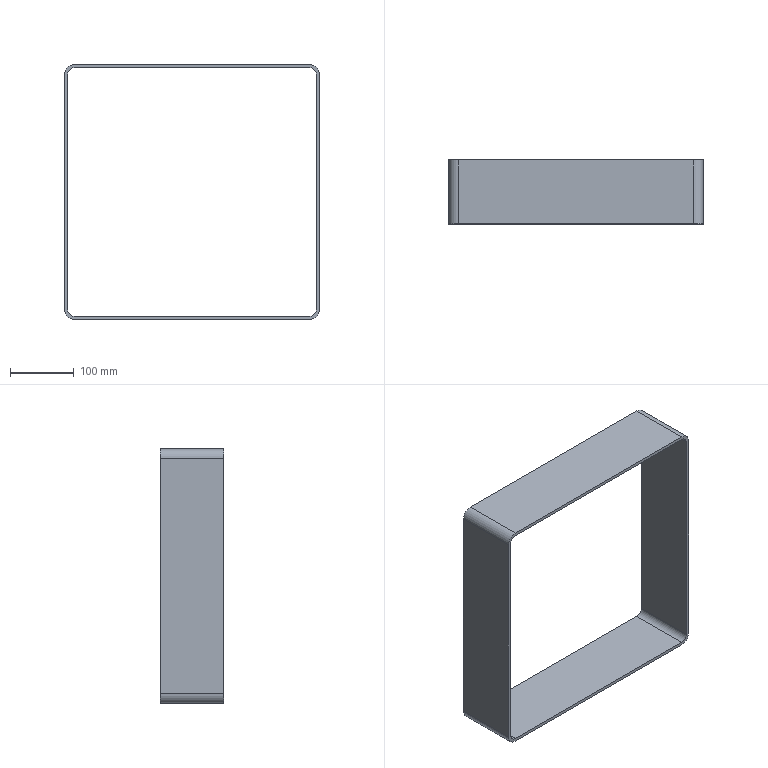Part | STEP file | Input 36 | 1 solid | 18 faces | box 400 x 100 x 400 mm | volume 779270 mm3 | plane 10 | cylinder 8 | commonest cylinder face diameters 20 x4 30 x4
STEP:
#1=CARTESIAN_POINT('',(0.,0.,0.));
#2=DIRECTION('',(0.,0.,1.));
#3=DIRECTION('',(1.,0.,0.));
#4=AXIS2_PLACEMENT_3D('',#1,#2,#3);
#5=CARTESIAN_POINT('',(-3055.,374.5,200.));
#6=VERTEX_POINT('',#5);
#7=CARTESIAN_POINT('',(-3040.,374.5,185.));
#8=VERTEX_POINT('',#7);
#9=CARTESIAN_POINT('',(-3055.,374.5,185.));
#10=DIRECTION('',(0.,1.,0.));
#11=DIRECTION('',(0.,0.,1.));
#12=AXIS2_PLACEMENT_3D('',#9,#10,#11);
#13=CIRCLE('',#12,15.);
#14=CARTESIAN_POINT('',(-3055.,374.5,185.));
#15=DIRECTION('',(0.,1.,0.));
#16=DIRECTION('',(0.,0.,1.));
#17=AXIS2_PLACEMENT_3D('',#14,#15,#16);
#18=PLANE('',#17);
#19=CARTESIAN_POINT('',(0.,0.));
#20=DIRECTION('',(1.,0.));
#21=AXIS2_PLACEMENT_2D('',#19,#20);
#22=CIRCLE('',#21,15.);
#23=(GEOMETRIC_REPRESENTATION_CONTEXT(2)PARAMETRIC_REPRESENTATION_CONTEXT()REPRESENTATION_CONTEXT('',''));
#24=DEFINITIONAL_REPRESENTATION('',(#22),#23);
#25=PCURVE('',#18,#24);
#26=CARTESIAN_POINT('',(-3055.,374.5,185.));
#27=DIRECTION('',(0.,-1.,0.));
#28=DIRECTION('',(0.,0.,-1.));
#29=AXIS2_PLACEMENT_3D('',#26,#27,#28);
#30=CYLINDRICAL_SURFACE('',#29,15.);
#31=CARTESIAN_POINT('',(3.142,0.));
#32=DIRECTION('',(-1.,0.));
#33=VECTOR('',#32,1.);
#34=LINE('',#31,#33);
#35=(GEOMETRIC_REPRESENTATION_CONTEXT(2)PARAMETRIC_REPRESENTATION_CONTEXT()REPRESENTATION_CONTEXT('',''));
#36=DEFINITIONAL_REPRESENTATION('',(#34),#35);
#37=PCURVE('',#30,#36);
#38=SURFACE_CURVE('',#13,(#25,#37),.PCURVE_S1.);
#39=EDGE_CURVE('',#6,#8,#38,.T.);
#40=ORIENTED_EDGE('',*,*,#39,.T.);
#41=CARTESIAN_POINT('',(-3040.,374.5,-185.));
#42=VERTEX_POINT('',#41);
#43=CARTESIAN_POINT('',(-3040.,374.5,185.));
#44=DIRECTION('',(0.,0.,-1.));
#45=VECTOR('',#44,1.);
#46=LINE('',#43,#45);
#47=CARTESIAN_POINT('',(0.,15.));
#48=DIRECTION('',(-1.,0.));
#49=VECTOR('',#48,1.);
#50=LINE('',#47,#49);
#51=(GEOMETRIC_REPRESENTATION_CONTEXT(2)PARAMETRIC_REPRESENTATION_CONTEXT()REPRESENTATION_CONTEXT('',''));
#52=DEFINITIONAL_REPRESENTATION('',(#50),#51);
#53=PCURVE('',#18,#52);
#54=CARTESIAN_POINT('',(-3040.,374.5,185.));
#55=DIRECTION('',(-1.,0.,0.));
#56=DIRECTION('',(0.,0.,1.));
#57=AXIS2_PLACEMENT_3D('',#54,#55,#56);
#58=PLANE('',#57);
#59=CARTESIAN_POINT('',(0.,0.));
#60=DIRECTION('',(-1.,0.));
#61=VECTOR('',#60,1.);
#62=LINE('',#59,#61);
#63=(GEOMETRIC_REPRESENTATION_CONTEXT(2)PARAMETRIC_REPRESENTATION_CONTEXT()REPRESENTATION_CONTEXT('',''));
#64=DEFINITIONAL_REPRESENTATION('',(#62),#63);
#65=PCURVE('',#58,#64);
#66=SURFACE_CURVE('',#46,(#53,#65),.PCURVE_S1.);
#67=EDGE_CURVE('',#8,#42,#66,.T.);
#68=ORIENTED_EDGE('',*,*,#67,.T.);
#69=CARTESIAN_POINT('',(-3055.,374.5,-200.));
#70=VERTEX_POINT('',#69);
#71=CARTESIAN_POINT('',(-3055.,374.5,-185.));
#72=DIRECTION('',(0.,1.,0.));
#73=DIRECTION('',(0.,0.,-1.));
#74=AXIS2_PLACEMENT_3D('',#71,#72,#73);
#75=CIRCLE('',#74,15.);
#76=CARTESIAN_POINT('',(-370.,0.));
#77=DIRECTION('',(-1.,0.));
#78=AXIS2_PLACEMENT_2D('',#76,#77);
#79=CIRCLE('',#78,15.);
#80=(GEOMETRIC_REPRESENTATION_CONTEXT(2)PARAMETRIC_REPRESENTATION_CONTEXT()REPRESENTATION_CONTEXT('',''));
#81=DEFINITIONAL_REPRESENTATION('',(#79),#80);
#82=PCURVE('',#18,#81);
#83=CARTESIAN_POINT('',(-3055.,374.5,-185.));
#84=DIRECTION('',(0.,-1.,0.));
#85=DIRECTION('',(0.,0.,-1.));
#86=AXIS2_PLACEMENT_3D('',#83,#84,#85);
#87=CYLINDRICAL_SURFACE('',#86,15.);
#88=CARTESIAN_POINT('',(6.283,0.));
#89=DIRECTION('',(-1.,0.));
#90=VECTOR('',#89,1.);
#91=LINE('',#88,#90);
#92=(GEOMETRIC_REPRESENTATION_CONTEXT(2)PARAMETRIC_REPRESENTATION_CONTEXT()REPRESENTATION_CONTEXT('',''));
#93=DEFINITIONAL_REPRESENTATION('',(#91),#92);
#94=PCURVE('',#87,#93);
#95=SURFACE_CURVE('',#75,(#82,#94),.PCURVE_S1.);
#96=EDGE_CURVE('',#42,#70,#95,.T.);
#97=ORIENTED_EDGE('',*,*,#96,.T.);
#98=CARTESIAN_POINT('',(-3425.,374.5,-200.));
#99=VERTEX_POINT('',#98);
#100=CARTESIAN_POINT('',(-3425.,374.5,-200.));
#101=DIRECTION('',(-1.,0.,0.));
#102=VECTOR('',#101,1.);
#103=LINE('',#100,#102);
#104=CARTESIAN_POINT('',(-385.,-370.));
#105=DIRECTION('',(0.,-1.));
#106=VECTOR('',#105,1.);
#107=LINE('',#104,#106);
#108=(GEOMETRIC_REPRESENTATION_CONTEXT(2)PARAMETRIC_REPRESENTATION_CONTEXT()REPRESENTATION_CONTEXT('',''));
#109=DEFINITIONAL_REPRESENTATION('',(#107),#108);
#110=PCURVE('',#18,#109);
#111=CARTESIAN_POINT('',(-3425.,374.5,-200.));
#112=DIRECTION('',(0.,0.,1.));
#113=DIRECTION('',(1.,0.,0.));
#114=AXIS2_PLACEMENT_3D('',#111,#112,#113);
#115=PLANE('',#114);
#116=CARTESIAN_POINT('',(0.,0.));
#117=DIRECTION('',(-1.,0.));
#118=VECTOR('',#117,1.);
#119=LINE('',#116,#118);
#120=(GEOMETRIC_REPRESENTATION_CONTEXT(2)PARAMETRIC_REPRESENTATION_CONTEXT()REPRESENTATION_CONTEXT('',''));
#121=DEFINITIONAL_REPRESENTATION('',(#119),#120);
#122=PCURVE('',#115,#121);
#123=SURFACE_CURVE('',#103,(#110,#122),.PCURVE_S1.);
#124=EDGE_CURVE('',#70,#99,#123,.T.);
#125=ORIENTED_EDGE('',*,*,#124,.T.);
#126=CARTESIAN_POINT('',(-3440.,374.5,-185.));
#127=VERTEX_POINT('',#126);
#128=CARTESIAN_POINT('',(-3425.,374.5,-185.));
#129=DIRECTION('',(0.,1.,0.));
#130=DIRECTION('',(0.,0.,-1.));
#131=AXIS2_PLACEMENT_3D('',#128,#129,#130);
#132=CIRCLE('',#131,15.);
#133=CARTESIAN_POINT('',(-370.,-370.));
#134=DIRECTION('',(-1.,0.));
#135=AXIS2_PLACEMENT_2D('',#133,#134);
#136=CIRCLE('',#135,15.);
#137=(GEOMETRIC_REPRESENTATION_CONTEXT(2)PARAMETRIC_REPRESENTATION_CONTEXT()REPRESENTATION_CONTEXT('',''));
#138=DEFINITIONAL_REPRESENTATION('',(#136),#137);
#139=PCURVE('',#18,#138);
#140=CARTESIAN_POINT('',(-3425.,374.5,-185.));
#141=DIRECTION('',(0.,-1.,0.));
#142=DIRECTION('',(0.,0.,-1.));
#143=AXIS2_PLACEMENT_3D('',#140,#141,#142);
#144=CYLINDRICAL_SURFACE('',#143,15.);
#145=CARTESIAN_POINT('',(6.283,0.));
#146=DIRECTION('',(-1.,0.));
#147=VECTOR('',#146,1.);
#148=LINE('',#145,#147);
#149=(GEOMETRIC_REPRESENTATION_CONTEXT(2)PARAMETRIC_REPRESENTATION_CONTEXT()REPRESENTATION_CONTEXT('',''));
#150=DEFINITIONAL_REPRESENTATION('',(#148),#149);
#151=PCURVE('',#144,#150);
#152=SURFACE_CURVE('',#132,(#139,#151),.PCURVE_S1.);
#153=EDGE_CURVE('',#99,#127,#152,.T.);
#154=ORIENTED_EDGE('',*,*,#153,.T.);
#155=CARTESIAN_POINT('',(-3440.,374.5,185.));
#156=VERTEX_POINT('',#155);
#157=CARTESIAN_POINT('',(-3440.,374.5,185.));
#158=DIRECTION('',(0.,0.,1.));
#159=VECTOR('',#158,1.);
#160=LINE('',#157,#159);
#161=CARTESIAN_POINT('',(0.,-385.));
#162=DIRECTION('',(1.,0.));
#163=VECTOR('',#162,1.);
#164=LINE('',#161,#163);
#165=(GEOMETRIC_REPRESENTATION_CONTEXT(2)PARAMETRIC_REPRESENTATION_CONTEXT()REPRESENTATION_CONTEXT('',''));
#166=DEFINITIONAL_REPRESENTATION('',(#164),#165);
#167=PCURVE('',#18,#166);
#168=CARTESIAN_POINT('',(-3440.,374.5,185.));
#169=DIRECTION('',(1.,0.,0.));
#170=DIRECTION('',(0.,0.,-1.));
#171=AXIS2_PLACEMENT_3D('',#168,#169,#170);
#172=PLANE('',#171);
#173=CARTESIAN_POINT('',(0.,0.));
#174=DIRECTION('',(-1.,0.));
#175=VECTOR('',#174,1.);
#176=LINE('',#173,#175);
#177=(GEOMETRIC_REPRESENTATION_CONTEXT(2)PARAMETRIC_REPRESENTATION_CONTEXT()REPRESENTATION_CONTEXT('',''));
#178=DEFINITIONAL_REPRESENTATION('',(#176),#177);
#179=PCURVE('',#172,#178);
#180=SURFACE_CURVE('',#160,(#167,#179),.PCURVE_S1.);
#181=EDGE_CURVE('',#127,#156,#180,.T.);
#182=ORIENTED_EDGE('',*,*,#181,.T.);
#183=CARTESIAN_POINT('',(-3425.,374.5,200.));
#184=VERTEX_POINT('',#183);
#185=CARTESIAN_POINT('',(-3425.,374.5,185.));
#186=DIRECTION('',(0.,1.,0.));
#187=DIRECTION('',(0.,0.,-1.));
#188=AXIS2_PLACEMENT_3D('',#185,#186,#187);
#189=CIRCLE('',#188,15.);
#190=CARTESIAN_POINT('',(0.,-370.));
#191=DIRECTION('',(-1.,0.));
#192=AXIS2_PLACEMENT_2D('',#190,#191);
#193=CIRCLE('',#192,15.);
#194=(GEOMETRIC_REPRESENTATION_CONTEXT(2)PARAMETRIC_REPRESENTATION_CONTEXT()REPRESENTATION_CONTEXT('',''));
#195=DEFINITIONAL_REPRESENTATION('',(#193),#194);
#196=PCURVE('',#18,#195);
#197=CARTESIAN_POINT('',(-3425.,374.5,185.));
#198=DIRECTION('',(0.,-1.,0.));
#199=DIRECTION('',(0.,0.,-1.));
#200=AXIS2_PLACEMENT_3D('',#197,#198,#199);
#201=CYLINDRICAL_SURFACE('',#200,15.);
#202=CARTESIAN_POINT('',(6.283,0.));
#203=DIRECTION('',(-1.,0.));
#204=VECTOR('',#203,1.);
#205=LINE('',#202,#204);
#206=(GEOMETRIC_REPRESENTATION_CONTEXT(2)PARAMETRIC_REPRESENTATION_CONTEXT()REPRESENTATION_CONTEXT('',''));
#207=DEFINITIONAL_REPRESENTATION('',(#205),#206);
#208=PCURVE('',#201,#207);
#209=SURFACE_CURVE('',#189,(#196,#208),.PCURVE_S1.);
#210=EDGE_CURVE('',#156,#184,#209,.T.);
#211=ORIENTED_EDGE('',*,*,#210,.T.);
#212=CARTESIAN_POINT('',(-3425.,374.5,200.));
#213=DIRECTION('',(1.,0.,0.));
#214=VECTOR('',#213,1.);
#215=LINE('',#212,#214);
#216=CARTESIAN_POINT('',(15.,-370.));
#217=DIRECTION('',(0.,1.));
#218=VECTOR('',#217,1.);
#219=LINE('',#216,#218);
#220=(GEOMETRIC_REPRESENTATION_CONTEXT(2)PARAMETRIC_REPRESENTATION_CONTEXT()REPRESENTATION_CONTEXT('',''));
#221=DEFINITIONAL_REPRESENTATION('',(#219),#220);
#222=PCURVE('',#18,#221);
#223=CARTESIAN_POINT('',(-3425.,374.5,200.));
#224=DIRECTION('',(0.,0.,-1.));
#225=DIRECTION('',(-1.,0.,0.));
#226=AXIS2_PLACEMENT_3D('',#223,#224,#225);
#227=PLANE('',#226);
#228=CARTESIAN_POINT('',(0.,0.));
#229=DIRECTION('',(-1.,0.));
#230=VECTOR('',#229,1.);
#231=LINE('',#228,#230);
#232=(GEOMETRIC_REPRESENTATION_CONTEXT(2)PARAMETRIC_REPRESENTATION_CONTEXT()REPRESENTATION_CONTEXT('',''));
#233=DEFINITIONAL_REPRESENTATION('',(#231),#232);
#234=PCURVE('',#227,#233);
#235=SURFACE_CURVE('',#215,(#222,#234),.PCURVE_S1.);
#236=EDGE_CURVE('',#184,#6,#235,.T.);
#237=ORIENTED_EDGE('',*,*,#236,.T.);
#238=EDGE_LOOP('',(#40,#68,#97,#125,#154,#182,#211,#237));
#239=FACE_BOUND('',#238,.T.);
#240=CARTESIAN_POINT('',(-3435.,374.5,-185.));
#241=VERTEX_POINT('',#240);
#242=CARTESIAN_POINT('',(-3435.,374.5,185.));
#243=VERTEX_POINT('',#242);
#244=CARTESIAN_POINT('',(-3435.,374.5,185.));
#245=DIRECTION('',(0.,0.,1.));
#246=VECTOR('',#245,1.);
#247=LINE('',#244,#246);
#248=CARTESIAN_POINT('',(0.,-380.));
#249=DIRECTION('',(1.,0.));
#250=VECTOR('',#249,1.);
#251=LINE('',#248,#250);
#252=(GEOMETRIC_REPRESENTATION_CONTEXT(2)PARAMETRIC_REPRESENTATION_CONTEXT()REPRESENTATION_CONTEXT('',''));
#253=DEFINITIONAL_REPRESENTATION('',(#251),#252);
#254=PCURVE('',#18,#253);
#255=CARTESIAN_POINT('',(-3435.,374.5,185.));
#256=DIRECTION('',(1.,0.,0.));
#257=DIRECTION('',(0.,0.,-1.));
#258=AXIS2_PLACEMENT_3D('',#255,#256,#257);
#259=PLANE('',#258);
#260=CARTESIAN_POINT('',(0.,0.));
#261=DIRECTION('',(-1.,0.));
#262=VECTOR('',#261,1.);
#263=LINE('',#260,#262);
#264=(GEOMETRIC_REPRESENTATION_CONTEXT(2)PARAMETRIC_REPRESENTATION_CONTEXT()REPRESENTATION_CONTEXT('',''));
#265=DEFINITIONAL_REPRESENTATION('',(#263),#264);
#266=PCURVE('',#259,#265);
#267=SURFACE_CURVE('',#247,(#254,#266),.PCURVE_S1.);
#268=EDGE_CURVE('',#241,#243,#267,.T.);
#269=ORIENTED_EDGE('',*,*,#268,.F.);
#270=CARTESIAN_POINT('',(-3425.,374.5,-195.));
#271=VERTEX_POINT('',#270);
#272=CARTESIAN_POINT('',(-3425.,374.5,-185.));
#273=DIRECTION('',(0.,1.,0.));
#274=DIRECTION('',(0.,0.,-1.));
#275=AXIS2_PLACEMENT_3D('',#272,#273,#274);
#276=CIRCLE('',#275,10.);
#277=CARTESIAN_POINT('',(-370.,-370.));
#278=DIRECTION('',(-1.,0.));
#279=AXIS2_PLACEMENT_2D('',#277,#278);
#280=CIRCLE('',#279,10.);
#281=(GEOMETRIC_REPRESENTATION_CONTEXT(2)PARAMETRIC_REPRESENTATION_CONTEXT()REPRESENTATION_CONTEXT('',''));
#282=DEFINITIONAL_REPRESENTATION('',(#280),#281);
#283=PCURVE('',#18,#282);
#284=CARTESIAN_POINT('',(-3425.,374.5,-185.));
#285=DIRECTION('',(0.,-1.,0.));
#286=DIRECTION('',(0.,0.,-1.));
#287=AXIS2_PLACEMENT_3D('',#284,#285,#286);
#288=CYLINDRICAL_SURFACE('',#287,10.);
#289=CARTESIAN_POINT('',(6.283,0.));
#290=DIRECTION('',(-1.,0.));
#291=VECTOR('',#290,1.);
#292=LINE('',#289,#291);
#293=(GEOMETRIC_REPRESENTATION_CONTEXT(2)PARAMETRIC_REPRESENTATION_CONTEXT()REPRESENTATION_CONTEXT('',''));
#294=DEFINITIONAL_REPRESENTATION('',(#292),#293);
#295=PCURVE('',#288,#294);
#296=SURFACE_CURVE('',#276,(#283,#295),.PCURVE_S1.);
#297=EDGE_CURVE('',#271,#241,#296,.T.);
#298=ORIENTED_EDGE('',*,*,#297,.F.);
#299=CARTESIAN_POINT('',(-3055.,374.5,-195.));
#300=VERTEX_POINT('',#299);
#301=CARTESIAN_POINT('',(-3425.,374.5,-195.));
#302=DIRECTION('',(-1.,0.,0.));
#303=VECTOR('',#302,1.);
#304=LINE('',#301,#303);
#305=CARTESIAN_POINT('',(-380.,-370.));
#306=DIRECTION('',(0.,-1.));
#307=VECTOR('',#306,1.);
#308=LINE('',#305,#307);
#309=(GEOMETRIC_REPRESENTATION_CONTEXT(2)PARAMETRIC_REPRESENTATION_CONTEXT()REPRESENTATION_CONTEXT('',''));
#310=DEFINITIONAL_REPRESENTATION('',(#308),#309);
#311=PCURVE('',#18,#310);
#312=CARTESIAN_POINT('',(-3425.,374.5,-195.));
#313=DIRECTION('',(0.,0.,1.));
#314=DIRECTION('',(1.,0.,0.));
#315=AXIS2_PLACEMENT_3D('',#312,#313,#314);
#316=PLANE('',#315);
#317=CARTESIAN_POINT('',(0.,0.));
#318=DIRECTION('',(-1.,0.));
#319=VECTOR('',#318,1.);
#320=LINE('',#317,#319);
#321=(GEOMETRIC_REPRESENTATION_CONTEXT(2)PARAMETRIC_REPRESENTATION_CONTEXT()REPRESENTATION_CONTEXT('',''));
#322=DEFINITIONAL_REPRESENTATION('',(#320),#321);
#323=PCURVE('',#316,#322);
#324=SURFACE_CURVE('',#304,(#311,#323),.PCURVE_S1.);
#325=EDGE_CURVE('',#300,#271,#324,.T.);
#326=ORIENTED_EDGE('',*,*,#325,.F.);
#327=CARTESIAN_POINT('',(-3045.,374.5,-185.));
#328=VERTEX_POINT('',#327);
#329=CARTESIAN_POINT('',(-3055.,374.5,-185.));
#330=DIRECTION('',(0.,1.,0.));
#331=DIRECTION('',(0.,0.,-1.));
#332=AXIS2_PLACEMENT_3D('',#329,#330,#331);
#333=CIRCLE('',#332,10.);
#334=CARTESIAN_POINT('',(-370.,0.));
#335=DIRECTION('',(-1.,0.));
#336=AXIS2_PLACEMENT_2D('',#334,#335);
#337=CIRCLE('',#336,10.);
#338=(GEOMETRIC_REPRESENTATION_CONTEXT(2)PARAMETRIC_REPRESENTATION_CONTEXT()REPRESENTATION_CONTEXT('',''));
#339=DEFINITIONAL_REPRESENTATION('',(#337),#338);
#340=PCURVE('',#18,#339);
#341=CARTESIAN_POINT('',(-3055.,374.5,-185.));
#342=DIRECTION('',(0.,-1.,0.));
#343=DIRECTION('',(0.,0.,-1.));
#344=AXIS2_PLACEMENT_3D('',#341,#342,#343);
#345=CYLINDRICAL_SURFACE('',#344,10.);
#346=CARTESIAN_POINT('',(6.283,0.));
#347=DIRECTION('',(-1.,0.));
#348=VECTOR('',#347,1.);
#349=LINE('',#346,#348);
#350=(GEOMETRIC_REPRESENTATION_CONTEXT(2)PARAMETRIC_REPRESENTATION_CONTEXT()REPRESENTATION_CONTEXT('',''));
#351=DEFINITIONAL_REPRESENTATION('',(#349),#350);
#352=PCURVE('',#345,#351);
#353=SURFACE_CURVE('',#333,(#340,#352),.PCURVE_S1.);
#354=EDGE_CURVE('',#328,#300,#353,.T.);
#355=ORIENTED_EDGE('',*,*,#354,.F.);
#356=CARTESIAN_POINT('',(-3045.,374.5,185.));
#357=VERTEX_POINT('',#356);
#358=CARTESIAN_POINT('',(-3045.,374.5,185.));
#359=DIRECTION('',(0.,0.,-1.));
#360=VECTOR('',#359,1.);
#361=LINE('',#358,#360);
#362=CARTESIAN_POINT('',(0.,10.));
#363=DIRECTION('',(-1.,0.));
#364=VECTOR('',#363,1.);
#365=LINE('',#362,#364);
#366=(GEOMETRIC_REPRESENTATION_CONTEXT(2)PARAMETRIC_REPRESENTATION_CONTEXT()REPRESENTATION_CONTEXT('',''));
#367=DEFINITIONAL_REPRESENTATION('',(#365),#366);
#368=PCURVE('',#18,#367);
#369=CARTESIAN_POINT('',(-3045.,374.5,185.));
#370=DIRECTION('',(-1.,0.,0.));
#371=DIRECTION('',(0.,0.,1.));
#372=AXIS2_PLACEMENT_3D('',#369,#370,#371);
#373=PLANE('',#372);
#374=CARTESIAN_POINT('',(0.,0.));
#375=DIRECTION('',(-1.,0.));
#376=VECTOR('',#375,1.);
#377=LINE('',#374,#376);
#378=(GEOMETRIC_REPRESENTATION_CONTEXT(2)PARAMETRIC_REPRESENTATION_CONTEXT()REPRESENTATION_CONTEXT('',''));
#379=DEFINITIONAL_REPRESENTATION('',(#377),#378);
#380=PCURVE('',#373,#379);
#381=SURFACE_CURVE('',#361,(#368,#380),.PCURVE_S1.);
#382=EDGE_CURVE('',#357,#328,#381,.T.);
#383=ORIENTED_EDGE('',*,*,#382,.F.);
#384=CARTESIAN_POINT('',(-3055.,374.5,195.));
#385=VERTEX_POINT('',#384);
#386=CARTESIAN_POINT('',(-3055.,374.5,185.));
#387=DIRECTION('',(0.,1.,0.));
#388=DIRECTION('',(0.,0.,1.));
#389=AXIS2_PLACEMENT_3D('',#386,#387,#388);
#390=CIRCLE('',#389,10.);
#391=CARTESIAN_POINT('',(0.,0.));
#392=DIRECTION('',(1.,0.));
#393=AXIS2_PLACEMENT_2D('',#391,#392);
#394=CIRCLE('',#393,10.);
#395=(GEOMETRIC_REPRESENTATION_CONTEXT(2)PARAMETRIC_REPRESENTATION_CONTEXT()REPRESENTATION_CONTEXT('',''));
#396=DEFINITIONAL_REPRESENTATION('',(#394),#395);
#397=PCURVE('',#18,#396);
#398=CARTESIAN_POINT('',(-3055.,374.5,185.));
#399=DIRECTION('',(0.,-1.,0.));
#400=DIRECTION('',(0.,0.,-1.));
#401=AXIS2_PLACEMENT_3D('',#398,#399,#400);
#402=CYLINDRICAL_SURFACE('',#401,10.);
#403=CARTESIAN_POINT('',(3.142,0.));
#404=DIRECTION('',(-1.,0.));
#405=VECTOR('',#404,1.);
#406=LINE('',#403,#405);
#407=(GEOMETRIC_REPRESENTATION_CONTEXT(2)PARAMETRIC_REPRESENTATION_CONTEXT()REPRESENTATION_CONTEXT('',''));
#408=DEFINITIONAL_REPRESENTATION('',(#406),#407);
#409=PCURVE('',#402,#408);
#410=SURFACE_CURVE('',#390,(#397,#409),.PCURVE_S1.);
#411=EDGE_CURVE('',#385,#357,#410,.T.);
#412=ORIENTED_EDGE('',*,*,#411,.F.);
#413=CARTESIAN_POINT('',(-3425.,374.5,195.));
#414=VERTEX_POINT('',#413);
#415=CARTESIAN_POINT('',(-3425.,374.5,195.));
#416=DIRECTION('',(1.,0.,0.));
#417=VECTOR('',#416,1.);
#418=LINE('',#415,#417);
#419=CARTESIAN_POINT('',(10.,-370.));
#420=DIRECTION('',(0.,1.));
#421=VECTOR('',#420,1.);
#422=LINE('',#419,#421);
#423=(GEOMETRIC_REPRESENTATION_CONTEXT(2)PARAMETRIC_REPRESENTATION_CONTEXT()REPRESENTATION_CONTEXT('',''));
#424=DEFINITIONAL_REPRESENTATION('',(#422),#423);
#425=PCURVE('',#18,#424);
#426=CARTESIAN_POINT('',(-3425.,374.5,195.));
#427=DIRECTION('',(0.,0.,-1.));
#428=DIRECTION('',(-1.,0.,0.));
#429=AXIS2_PLACEMENT_3D('',#426,#427,#428);
#430=PLANE('',#429);
#431=CARTESIAN_POINT('',(0.,0.));
#432=DIRECTION('',(-1.,0.));
#433=VECTOR('',#432,1.);
#434=LINE('',#431,#433);
#435=(GEOMETRIC_REPRESENTATION_CONTEXT(2)PARAMETRIC_REPRESENTATION_CONTEXT()REPRESENTATION_CONTEXT('',''));
#436=DEFINITIONAL_REPRESENTATION('',(#434),#435);
#437=PCURVE('',#430,#436);
#438=SURFACE_CURVE('',#418,(#425,#437),.PCURVE_S1.);
#439=EDGE_CURVE('',#414,#385,#438,.T.);
#440=ORIENTED_EDGE('',*,*,#439,.F.);
#441=CARTESIAN_POINT('',(-3425.,374.5,185.));
#442=DIRECTION('',(0.,1.,0.));
#443=DIRECTION('',(0.,0.,-1.));
#444=AXIS2_PLACEMENT_3D('',#441,#442,#443);
#445=CIRCLE('',#444,10.);
#446=CARTESIAN_POINT('',(0.,-370.));
#447=DIRECTION('',(-1.,0.));
#448=AXIS2_PLACEMENT_2D('',#446,#447);
#449=CIRCLE('',#448,10.);
#450=(GEOMETRIC_REPRESENTATION_CONTEXT(2)PARAMETRIC_REPRESENTATION_CONTEXT()REPRESENTATION_CONTEXT('',''));
#451=DEFINITIONAL_REPRESENTATION('',(#449),#450);
#452=PCURVE('',#18,#451);
#453=CARTESIAN_POINT('',(-3425.,374.5,185.));
#454=DIRECTION('',(0.,-1.,0.));
#455=DIRECTION('',(0.,0.,-1.));
#456=AXIS2_PLACEMENT_3D('',#453,#454,#455);
#457=CYLINDRICAL_SURFACE('',#456,10.);
#458=CARTESIAN_POINT('',(6.283,0.));
#459=DIRECTION('',(-1.,0.));
#460=VECTOR('',#459,1.);
#461=LINE('',#458,#460);
#462=(GEOMETRIC_REPRESENTATION_CONTEXT(2)PARAMETRIC_REPRESENTATION_CONTEXT()REPRESENTATION_CONTEXT('',''));
#463=DEFINITIONAL_REPRESENTATION('',(#461),#462);
#464=PCURVE('',#457,#463);
#465=SURFACE_CURVE('',#445,(#452,#464),.PCURVE_S1.);
#466=EDGE_CURVE('',#243,#414,#465,.T.);
#467=ORIENTED_EDGE('',*,*,#466,.F.);
#468=EDGE_LOOP('',(#269,#298,#326,#355,#383,#412,#440,#467));
#469=FACE_BOUND('',#468,.T.);
#470=ADVANCED_FACE('',(#239,#469),#18,.T.);
#471=CARTESIAN_POINT('',(-3055.,274.5,200.));
#472=VERTEX_POINT('',#471);
#473=CARTESIAN_POINT('',(-3040.,274.5,185.));
#474=VERTEX_POINT('',#473);
#475=CARTESIAN_POINT('',(-3055.,274.5,185.));
#476=DIRECTION('',(0.,1.,0.));
#477=DIRECTION('',(0.,0.,1.));
#478=AXIS2_PLACEMENT_3D('',#475,#476,#477);
#479=CIRCLE('',#478,15.);
#480=CARTESIAN_POINT('',(-3055.,274.5,185.));
#481=DIRECTION('',(0.,1.,0.));
#482=DIRECTION('',(0.,0.,1.));
#483=AXIS2_PLACEMENT_3D('',#480,#481,#482);
#484=PLANE('',#483);
#485=CARTESIAN_POINT('',(0.,0.));
#486=DIRECTION('',(1.,0.));
#487=AXIS2_PLACEMENT_2D('',#485,#486);
#488=CIRCLE('',#487,15.);
#489=(GEOMETRIC_REPRESENTATION_CONTEXT(2)PARAMETRIC_REPRESENTATION_CONTEXT()REPRESENTATION_CONTEXT('',''));
#490=DEFINITIONAL_REPRESENTATION('',(#488),#489);
#491=PCURVE('',#484,#490);
#492=CARTESIAN_POINT('',(3.142,100.));
#493=DIRECTION('',(-1.,0.));
#494=VECTOR('',#493,1.);
#495=LINE('',#492,#494);
#496=(GEOMETRIC_REPRESENTATION_CONTEXT(2)PARAMETRIC_REPRESENTATION_CONTEXT()REPRESENTATION_CONTEXT('',''));
#497=DEFINITIONAL_REPRESENTATION('',(#495),#496);
#498=PCURVE('',#30,#497);
#499=SURFACE_CURVE('',#479,(#491,#498),.PCURVE_S1.);
#500=EDGE_CURVE('',#472,#474,#499,.T.);
#501=ORIENTED_EDGE('',*,*,#500,.F.);
#502=CARTESIAN_POINT('',(-3425.,274.5,200.));
#503=VERTEX_POINT('',#502);
#504=CARTESIAN_POINT('',(-3425.,274.5,200.));
#505=DIRECTION('',(1.,0.,0.));
#506=VECTOR('',#505,1.);
#507=LINE('',#504,#506);
#508=CARTESIAN_POINT('',(15.,-370.));
#509=DIRECTION('',(0.,1.));
#510=VECTOR('',#509,1.);
#511=LINE('',#508,#510);
#512=(GEOMETRIC_REPRESENTATION_CONTEXT(2)PARAMETRIC_REPRESENTATION_CONTEXT()REPRESENTATION_CONTEXT('',''));
#513=DEFINITIONAL_REPRESENTATION('',(#511),#512);
#514=PCURVE('',#484,#513);
#515=CARTESIAN_POINT('',(0.,-100.));
#516=DIRECTION('',(-1.,0.));
#517=VECTOR('',#516,1.);
#518=LINE('',#515,#517);
#519=(GEOMETRIC_REPRESENTATION_CONTEXT(2)PARAMETRIC_REPRESENTATION_CONTEXT()REPRESENTATION_CONTEXT('',''));
#520=DEFINITIONAL_REPRESENTATION('',(#518),#519);
#521=PCURVE('',#227,#520);
#522=SURFACE_CURVE('',#507,(#514,#521),.PCURVE_S1.);
#523=EDGE_CURVE('',#503,#472,#522,.T.);
#524=ORIENTED_EDGE('',*,*,#523,.F.);
#525=CARTESIAN_POINT('',(-3440.,274.5,185.));
#526=VERTEX_POINT('',#525);
#527=CARTESIAN_POINT('',(-3425.,274.5,185.));
#528=DIRECTION('',(0.,1.,0.));
#529=DIRECTION('',(0.,0.,-1.));
#530=AXIS2_PLACEMENT_3D('',#527,#528,#529);
#531=CIRCLE('',#530,15.);
#532=CARTESIAN_POINT('',(0.,-370.));
#533=DIRECTION('',(-1.,0.));
#534=AXIS2_PLACEMENT_2D('',#532,#533);
#535=CIRCLE('',#534,15.);
#536=(GEOMETRIC_REPRESENTATION_CONTEXT(2)PARAMETRIC_REPRESENTATION_CONTEXT()REPRESENTATION_CONTEXT('',''));
#537=DEFINITIONAL_REPRESENTATION('',(#535),#536);
#538=PCURVE('',#484,#537);
#539=CARTESIAN_POINT('',(6.283,100.));
#540=DIRECTION('',(-1.,0.));
#541=VECTOR('',#540,1.);
#542=LINE('',#539,#541);
#543=(GEOMETRIC_REPRESENTATION_CONTEXT(2)PARAMETRIC_REPRESENTATION_CONTEXT()REPRESENTATION_CONTEXT('',''));
#544=DEFINITIONAL_REPRESENTATION('',(#542),#543);
#545=PCURVE('',#201,#544);
#546=SURFACE_CURVE('',#531,(#538,#545),.PCURVE_S1.);
#547=EDGE_CURVE('',#526,#503,#546,.T.);
#548=ORIENTED_EDGE('',*,*,#547,.F.);
#549=CARTESIAN_POINT('',(-3440.,274.5,-185.));
#550=VERTEX_POINT('',#549);
#551=CARTESIAN_POINT('',(-3440.,274.5,185.));
#552=DIRECTION('',(0.,0.,1.));
#553=VECTOR('',#552,1.);
#554=LINE('',#551,#553);
#555=CARTESIAN_POINT('',(0.,-385.));
#556=DIRECTION('',(1.,0.));
#557=VECTOR('',#556,1.);
#558=LINE('',#555,#557);
#559=(GEOMETRIC_REPRESENTATION_CONTEXT(2)PARAMETRIC_REPRESENTATION_CONTEXT()REPRESENTATION_CONTEXT('',''));
#560=DEFINITIONAL_REPRESENTATION('',(#558),#559);
#561=PCURVE('',#484,#560);
#562=CARTESIAN_POINT('',(0.,-100.));
#563=DIRECTION('',(-1.,0.));
#564=VECTOR('',#563,1.);
#565=LINE('',#562,#564);
#566=(GEOMETRIC_REPRESENTATION_CONTEXT(2)PARAMETRIC_REPRESENTATION_CONTEXT()REPRESENTATION_CONTEXT('',''));
#567=DEFINITIONAL_REPRESENTATION('',(#565),#566);
#568=PCURVE('',#172,#567);
#569=SURFACE_CURVE('',#554,(#561,#568),.PCURVE_S1.);
#570=EDGE_CURVE('',#550,#526,#569,.T.);
#571=ORIENTED_EDGE('',*,*,#570,.F.);
#572=CARTESIAN_POINT('',(-3425.,274.5,-200.));
#573=VERTEX_POINT('',#572);
#574=CARTESIAN_POINT('',(-3425.,274.5,-185.));
#575=DIRECTION('',(0.,1.,0.));
#576=DIRECTION('',(0.,0.,-1.));
#577=AXIS2_PLACEMENT_3D('',#574,#575,#576);
#578=CIRCLE('',#577,15.);
#579=CARTESIAN_POINT('',(-370.,-370.));
#580=DIRECTION('',(-1.,0.));
#581=AXIS2_PLACEMENT_2D('',#579,#580);
#582=CIRCLE('',#581,15.);
#583=(GEOMETRIC_REPRESENTATION_CONTEXT(2)PARAMETRIC_REPRESENTATION_CONTEXT()REPRESENTATION_CONTEXT('',''));
#584=DEFINITIONAL_REPRESENTATION('',(#582),#583);
#585=PCURVE('',#484,#584);
#586=CARTESIAN_POINT('',(6.283,100.));
#587=DIRECTION('',(-1.,0.));
#588=VECTOR('',#587,1.);
#589=LINE('',#586,#588);
#590=(GEOMETRIC_REPRESENTATION_CONTEXT(2)PARAMETRIC_REPRESENTATION_CONTEXT()REPRESENTATION_CONTEXT('',''));
#591=DEFINITIONAL_REPRESENTATION('',(#589),#590);
#592=PCURVE('',#144,#591);
#593=SURFACE_CURVE('',#578,(#585,#592),.PCURVE_S1.);
#594=EDGE_CURVE('',#573,#550,#593,.T.);
#595=ORIENTED_EDGE('',*,*,#594,.F.);
#596=CARTESIAN_POINT('',(-3055.,274.5,-200.));
#597=VERTEX_POINT('',#596);
#598=CARTESIAN_POINT('',(-3425.,274.5,-200.));
#599=DIRECTION('',(-1.,0.,0.));
#600=VECTOR('',#599,1.);
#601=LINE('',#598,#600);
#602=CARTESIAN_POINT('',(-385.,-370.));
#603=DIRECTION('',(0.,-1.));
#604=VECTOR('',#603,1.);
#605=LINE('',#602,#604);
#606=(GEOMETRIC_REPRESENTATION_CONTEXT(2)PARAMETRIC_REPRESENTATION_CONTEXT()REPRESENTATION_CONTEXT('',''));
#607=DEFINITIONAL_REPRESENTATION('',(#605),#606);
#608=PCURVE('',#484,#607);
#609=CARTESIAN_POINT('',(0.,-100.));
#610=DIRECTION('',(-1.,0.));
#611=VECTOR('',#610,1.);
#612=LINE('',#609,#611);
#613=(GEOMETRIC_REPRESENTATION_CONTEXT(2)PARAMETRIC_REPRESENTATION_CONTEXT()REPRESENTATION_CONTEXT('',''));
#614=DEFINITIONAL_REPRESENTATION('',(#612),#613);
#615=PCURVE('',#115,#614);
#616=SURFACE_CURVE('',#601,(#608,#615),.PCURVE_S1.);
#617=EDGE_CURVE('',#597,#573,#616,.T.);
#618=ORIENTED_EDGE('',*,*,#617,.F.);
#619=CARTESIAN_POINT('',(-3040.,274.5,-185.));
#620=VERTEX_POINT('',#619);
#621=CARTESIAN_POINT('',(-3055.,274.5,-185.));
#622=DIRECTION('',(0.,1.,0.));
#623=DIRECTION('',(0.,0.,-1.));
#624=AXIS2_PLACEMENT_3D('',#621,#622,#623);
#625=CIRCLE('',#624,15.);
#626=CARTESIAN_POINT('',(-370.,0.));
#627=DIRECTION('',(-1.,0.));
#628=AXIS2_PLACEMENT_2D('',#626,#627);
#629=CIRCLE('',#628,15.);
#630=(GEOMETRIC_REPRESENTATION_CONTEXT(2)PARAMETRIC_REPRESENTATION_CONTEXT()REPRESENTATION_CONTEXT('',''));
#631=DEFINITIONAL_REPRESENTATION('',(#629),#630);
#632=PCURVE('',#484,#631);
#633=CARTESIAN_POINT('',(6.283,100.));
#634=DIRECTION('',(-1.,0.));
#635=VECTOR('',#634,1.);
#636=LINE('',#633,#635);
#637=(GEOMETRIC_REPRESENTATION_CONTEXT(2)PARAMETRIC_REPRESENTATION_CONTEXT()REPRESENTATION_CONTEXT('',''));
#638=DEFINITIONAL_REPRESENTATION('',(#636),#637);
#639=PCURVE('',#87,#638);
#640=SURFACE_CURVE('',#625,(#632,#639),.PCURVE_S1.);
#641=EDGE_CURVE('',#620,#597,#640,.T.);
#642=ORIENTED_EDGE('',*,*,#641,.F.);
#643=CARTESIAN_POINT('',(-3040.,274.5,185.));
#644=DIRECTION('',(0.,0.,-1.));
#645=VECTOR('',#644,1.);
#646=LINE('',#643,#645);
#647=CARTESIAN_POINT('',(0.,15.));
#648=DIRECTION('',(-1.,0.));
#649=VECTOR('',#648,1.);
#650=LINE('',#647,#649);
#651=(GEOMETRIC_REPRESENTATION_CONTEXT(2)PARAMETRIC_REPRESENTATION_CONTEXT()REPRESENTATION_CONTEXT('',''));
#652=DEFINITIONAL_REPRESENTATION('',(#650),#651);
#653=PCURVE('',#484,#652);
#654=CARTESIAN_POINT('',(0.,-100.));
#655=DIRECTION('',(-1.,0.));
#656=VECTOR('',#655,1.);
#657=LINE('',#654,#656);
#658=(GEOMETRIC_REPRESENTATION_CONTEXT(2)PARAMETRIC_REPRESENTATION_CONTEXT()REPRESENTATION_CONTEXT('',''));
#659=DEFINITIONAL_REPRESENTATION('',(#657),#658);
#660=PCURVE('',#58,#659);
#661=SURFACE_CURVE('',#646,(#653,#660),.PCURVE_S1.);
#662=EDGE_CURVE('',#474,#620,#661,.T.);
#663=ORIENTED_EDGE('',*,*,#662,.F.);
#664=EDGE_LOOP('',(#501,#524,#548,#571,#595,#618,#642,#663));
#665=FACE_BOUND('',#664,.T.);
#666=CARTESIAN_POINT('',(-3425.,274.5,-195.));
#667=VERTEX_POINT('',#666);
#668=CARTESIAN_POINT('',(-3435.,274.5,-185.));
#669=VERTEX_POINT('',#668);
#670=CARTESIAN_POINT('',(-3425.,274.5,-185.));
#671=DIRECTION('',(0.,1.,0.));
#672=DIRECTION('',(0.,0.,-1.));
#673=AXIS2_PLACEMENT_3D('',#670,#671,#672);
#674=CIRCLE('',#673,10.);
#675=CARTESIAN_POINT('',(-370.,-370.));
#676=DIRECTION('',(-1.,0.));
#677=AXIS2_PLACEMENT_2D('',#675,#676);
#678=CIRCLE('',#677,10.);
#679=(GEOMETRIC_REPRESENTATION_CONTEXT(2)PARAMETRIC_REPRESENTATION_CONTEXT()REPRESENTATION_CONTEXT('',''));
#680=DEFINITIONAL_REPRESENTATION('',(#678),#679);
#681=PCURVE('',#484,#680);
#682=CARTESIAN_POINT('',(6.283,100.));
#683=DIRECTION('',(-1.,0.));
#684=VECTOR('',#683,1.);
#685=LINE('',#682,#684);
#686=(GEOMETRIC_REPRESENTATION_CONTEXT(2)PARAMETRIC_REPRESENTATION_CONTEXT()REPRESENTATION_CONTEXT('',''));
#687=DEFINITIONAL_REPRESENTATION('',(#685),#686);
#688=PCURVE('',#288,#687);
#689=SURFACE_CURVE('',#674,(#681,#688),.PCURVE_S1.);
#690=EDGE_CURVE('',#667,#669,#689,.T.);
#691=ORIENTED_EDGE('',*,*,#690,.T.);
#692=CARTESIAN_POINT('',(-3435.,274.5,185.));
#693=VERTEX_POINT('',#692);
#694=CARTESIAN_POINT('',(-3435.,274.5,185.));
#695=DIRECTION('',(0.,0.,1.));
#696=VECTOR('',#695,1.);
#697=LINE('',#694,#696);
#698=CARTESIAN_POINT('',(0.,-380.));
#699=DIRECTION('',(1.,0.));
#700=VECTOR('',#699,1.);
#701=LINE('',#698,#700);
#702=(GEOMETRIC_REPRESENTATION_CONTEXT(2)PARAMETRIC_REPRESENTATION_CONTEXT()REPRESENTATION_CONTEXT('',''));
#703=DEFINITIONAL_REPRESENTATION('',(#701),#702);
#704=PCURVE('',#484,#703);
#705=CARTESIAN_POINT('',(0.,-100.));
#706=DIRECTION('',(-1.,0.));
#707=VECTOR('',#706,1.);
#708=LINE('',#705,#707);
#709=(GEOMETRIC_REPRESENTATION_CONTEXT(2)PARAMETRIC_REPRESENTATION_CONTEXT()REPRESENTATION_CONTEXT('',''));
#710=DEFINITIONAL_REPRESENTATION('',(#708),#709);
#711=PCURVE('',#259,#710);
#712=SURFACE_CURVE('',#697,(#704,#711),.PCURVE_S1.);
#713=EDGE_CURVE('',#669,#693,#712,.T.);
#714=ORIENTED_EDGE('',*,*,#713,.T.);
#715=CARTESIAN_POINT('',(-3425.,274.5,195.));
#716=VERTEX_POINT('',#715);
#717=CARTESIAN_POINT('',(-3425.,274.5,185.));
#718=DIRECTION('',(0.,1.,0.));
#719=DIRECTION('',(0.,0.,-1.));
#720=AXIS2_PLACEMENT_3D('',#717,#718,#719);
#721=CIRCLE('',#720,10.);
#722=CARTESIAN_POINT('',(0.,-370.));
#723=DIRECTION('',(-1.,0.));
#724=AXIS2_PLACEMENT_2D('',#722,#723);
#725=CIRCLE('',#724,10.);
#726=(GEOMETRIC_REPRESENTATION_CONTEXT(2)PARAMETRIC_REPRESENTATION_CONTEXT()REPRESENTATION_CONTEXT('',''));
#727=DEFINITIONAL_REPRESENTATION('',(#725),#726);
#728=PCURVE('',#484,#727);
#729=CARTESIAN_POINT('',(6.283,100.));
#730=DIRECTION('',(-1.,0.));
#731=VECTOR('',#730,1.);
#732=LINE('',#729,#731);
#733=(GEOMETRIC_REPRESENTATION_CONTEXT(2)PARAMETRIC_REPRESENTATION_CONTEXT()REPRESENTATION_CONTEXT('',''));
#734=DEFINITIONAL_REPRESENTATION('',(#732),#733);
#735=PCURVE('',#457,#734);
#736=SURFACE_CURVE('',#721,(#728,#735),.PCURVE_S1.);
#737=EDGE_CURVE('',#693,#716,#736,.T.);
#738=ORIENTED_EDGE('',*,*,#737,.T.);
#739=CARTESIAN_POINT('',(-3055.,274.5,195.));
#740=VERTEX_POINT('',#739);
#741=CARTESIAN_POINT('',(-3425.,274.5,195.));
#742=DIRECTION('',(1.,0.,0.));
#743=VECTOR('',#742,1.);
#744=LINE('',#741,#743);
#745=CARTESIAN_POINT('',(10.,-370.));
#746=DIRECTION('',(0.,1.));
#747=VECTOR('',#746,1.);
#748=LINE('',#745,#747);
#749=(GEOMETRIC_REPRESENTATION_CONTEXT(2)PARAMETRIC_REPRESENTATION_CONTEXT()REPRESENTATION_CONTEXT('',''));
#750=DEFINITIONAL_REPRESENTATION('',(#748),#749);
#751=PCURVE('',#484,#750);
#752=CARTESIAN_POINT('',(0.,-100.));
#753=DIRECTION('',(-1.,0.));
#754=VECTOR('',#753,1.);
#755=LINE('',#752,#754);
#756=(GEOMETRIC_REPRESENTATION_CONTEXT(2)PARAMETRIC_REPRESENTATION_CONTEXT()REPRESENTATION_CONTEXT('',''));
#757=DEFINITIONAL_REPRESENTATION('',(#755),#756);
#758=PCURVE('',#430,#757);
#759=SURFACE_CURVE('',#744,(#751,#758),.PCURVE_S1.);
#760=EDGE_CURVE('',#716,#740,#759,.T.);
#761=ORIENTED_EDGE('',*,*,#760,.T.);
#762=CARTESIAN_POINT('',(-3045.,274.5,185.));
#763=VERTEX_POINT('',#762);
#764=CARTESIAN_POINT('',(-3055.,274.5,185.));
#765=DIRECTION('',(0.,1.,0.));
#766=DIRECTION('',(0.,0.,1.));
#767=AXIS2_PLACEMENT_3D('',#764,#765,#766);
#768=CIRCLE('',#767,10.);
#769=CARTESIAN_POINT('',(0.,0.));
#770=DIRECTION('',(1.,0.));
#771=AXIS2_PLACEMENT_2D('',#769,#770);
#772=CIRCLE('',#771,10.);
#773=(GEOMETRIC_REPRESENTATION_CONTEXT(2)PARAMETRIC_REPRESENTATION_CONTEXT()REPRESENTATION_CONTEXT('',''));
#774=DEFINITIONAL_REPRESENTATION('',(#772),#773);
#775=PCURVE('',#484,#774);
#776=CARTESIAN_POINT('',(3.142,100.));
#777=DIRECTION('',(-1.,0.));
#778=VECTOR('',#777,1.);
#779=LINE('',#776,#778);
#780=(GEOMETRIC_REPRESENTATION_CONTEXT(2)PARAMETRIC_REPRESENTATION_CONTEXT()REPRESENTATION_CONTEXT('',''));
#781=DEFINITIONAL_REPRESENTATION('',(#779),#780);
#782=PCURVE('',#402,#781);
#783=SURFACE_CURVE('',#768,(#775,#782),.PCURVE_S1.);
#784=EDGE_CURVE('',#740,#763,#783,.T.);
#785=ORIENTED_EDGE('',*,*,#784,.T.);
#786=CARTESIAN_POINT('',(-3045.,274.5,-185.));
#787=VERTEX_POINT('',#786);
#788=CARTESIAN_POINT('',(-3045.,274.5,185.));
#789=DIRECTION('',(0.,0.,-1.));
#790=VECTOR('',#789,1.);
#791=LINE('',#788,#790);
#792=CARTESIAN_POINT('',(0.,10.));
#793=DIRECTION('',(-1.,0.));
#794=VECTOR('',#793,1.);
#795=LINE('',#792,#794);
#796=(GEOMETRIC_REPRESENTATION_CONTEXT(2)PARAMETRIC_REPRESENTATION_CONTEXT()REPRESENTATION_CONTEXT('',''));
#797=DEFINITIONAL_REPRESENTATION('',(#795),#796);
#798=PCURVE('',#484,#797);
#799=CARTESIAN_POINT('',(0.,-100.));
#800=DIRECTION('',(-1.,0.));
#801=VECTOR('',#800,1.);
#802=LINE('',#799,#801);
#803=(GEOMETRIC_REPRESENTATION_CONTEXT(2)PARAMETRIC_REPRESENTATION_CONTEXT()REPRESENTATION_CONTEXT('',''));
#804=DEFINITIONAL_REPRESENTATION('',(#802),#803);
#805=PCURVE('',#373,#804);
#806=SURFACE_CURVE('',#791,(#798,#805),.PCURVE_S1.);
#807=EDGE_CURVE('',#763,#787,#806,.T.);
#808=ORIENTED_EDGE('',*,*,#807,.T.);
#809=CARTESIAN_POINT('',(-3055.,274.5,-195.));
#810=VERTEX_POINT('',#809);
#811=CARTESIAN_POINT('',(-3055.,274.5,-185.));
#812=DIRECTION('',(0.,1.,0.));
#813=DIRECTION('',(0.,0.,-1.));
#814=AXIS2_PLACEMENT_3D('',#811,#812,#813);
#815=CIRCLE('',#814,10.);
#816=CARTESIAN_POINT('',(-370.,0.));
#817=DIRECTION('',(-1.,0.));
#818=AXIS2_PLACEMENT_2D('',#816,#817);
#819=CIRCLE('',#818,10.);
#820=(GEOMETRIC_REPRESENTATION_CONTEXT(2)PARAMETRIC_REPRESENTATION_CONTEXT()REPRESENTATION_CONTEXT('',''));
#821=DEFINITIONAL_REPRESENTATION('',(#819),#820);
#822=PCURVE('',#484,#821);
#823=CARTESIAN_POINT('',(6.283,100.));
#824=DIRECTION('',(-1.,0.));
#825=VECTOR('',#824,1.);
#826=LINE('',#823,#825);
#827=(GEOMETRIC_REPRESENTATION_CONTEXT(2)PARAMETRIC_REPRESENTATION_CONTEXT()REPRESENTATION_CONTEXT('',''));
#828=DEFINITIONAL_REPRESENTATION('',(#826),#827);
#829=PCURVE('',#345,#828);
#830=SURFACE_CURVE('',#815,(#822,#829),.PCURVE_S1.);
#831=EDGE_CURVE('',#787,#810,#830,.T.);
#832=ORIENTED_EDGE('',*,*,#831,.T.);
#833=CARTESIAN_POINT('',(-3425.,274.5,-195.));
#834=DIRECTION('',(-1.,0.,0.));
#835=VECTOR('',#834,1.);
#836=LINE('',#833,#835);
#837=CARTESIAN_POINT('',(-380.,-370.));
#838=DIRECTION('',(0.,-1.));
#839=VECTOR('',#838,1.);
#840=LINE('',#837,#839);
#841=(GEOMETRIC_REPRESENTATION_CONTEXT(2)PARAMETRIC_REPRESENTATION_CONTEXT()REPRESENTATION_CONTEXT('',''));
#842=DEFINITIONAL_REPRESENTATION('',(#840),#841);
#843=PCURVE('',#484,#842);
#844=CARTESIAN_POINT('',(0.,-100.));
#845=DIRECTION('',(-1.,0.));
#846=VECTOR('',#845,1.);
#847=LINE('',#844,#846);
#848=(GEOMETRIC_REPRESENTATION_CONTEXT(2)PARAMETRIC_REPRESENTATION_CONTEXT()REPRESENTATION_CONTEXT('',''));
#849=DEFINITIONAL_REPRESENTATION('',(#847),#848);
#850=PCURVE('',#316,#849);
#851=SURFACE_CURVE('',#836,(#843,#850),.PCURVE_S1.);
#852=EDGE_CURVE('',#810,#667,#851,.T.);
#853=ORIENTED_EDGE('',*,*,#852,.T.);
#854=EDGE_LOOP('',(#691,#714,#738,#761,#785,#808,#832,#853));
#855=FACE_BOUND('',#854,.T.);
#856=ADVANCED_FACE('',(#665,#855),#484,.F.);
#857=ORIENTED_EDGE('',*,*,#500,.T.);
#858=CARTESIAN_POINT('',(-3040.,374.5,185.));
#859=DIRECTION('',(0.,-1.,0.));
#860=VECTOR('',#859,1.);
#861=LINE('',#858,#860);
#862=CARTESIAN_POINT('',(1.571,0.));
#863=DIRECTION('',(0.,1.));
#864=VECTOR('',#863,1.);
#865=LINE('',#862,#864);
#866=(GEOMETRIC_REPRESENTATION_CONTEXT(2)PARAMETRIC_REPRESENTATION_CONTEXT()REPRESENTATION_CONTEXT('',''));
#867=DEFINITIONAL_REPRESENTATION('',(#865),#866);
#868=PCURVE('',#30,#867);
#869=CARTESIAN_POINT('',(0.,0.));
#870=DIRECTION('',(0.,-1.));
#871=VECTOR('',#870,1.);
#872=LINE('',#869,#871);
#873=(GEOMETRIC_REPRESENTATION_CONTEXT(2)PARAMETRIC_REPRESENTATION_CONTEXT()REPRESENTATION_CONTEXT('',''));
#874=DEFINITIONAL_REPRESENTATION('',(#872),#873);
#875=PCURVE('',#58,#874);
#876=SURFACE_CURVE('',#861,(#868,#875),.PCURVE_S1.);
#877=EDGE_CURVE('',#8,#474,#876,.T.);
#878=ORIENTED_EDGE('',*,*,#877,.F.);
#879=ORIENTED_EDGE('',*,*,#39,.F.);
#880=CARTESIAN_POINT('',(-3055.,374.5,200.));
#881=DIRECTION('',(0.,-1.,0.));
#882=VECTOR('',#881,1.);
#883=LINE('',#880,#882);
#884=CARTESIAN_POINT('',(3.142,0.));
#885=DIRECTION('',(0.,1.));
#886=VECTOR('',#885,1.);
#887=LINE('',#884,#886);
#888=(GEOMETRIC_REPRESENTATION_CONTEXT(2)PARAMETRIC_REPRESENTATION_CONTEXT()REPRESENTATION_CONTEXT('',''));
#889=DEFINITIONAL_REPRESENTATION('',(#887),#888);
#890=PCURVE('',#30,#889);
#891=CARTESIAN_POINT('',(-370.,0.));
#892=DIRECTION('',(0.,-1.));
#893=VECTOR('',#892,1.);
#894=LINE('',#891,#893);
#895=(GEOMETRIC_REPRESENTATION_CONTEXT(2)PARAMETRIC_REPRESENTATION_CONTEXT()REPRESENTATION_CONTEXT('',''));
#896=DEFINITIONAL_REPRESENTATION('',(#894),#895);
#897=PCURVE('',#227,#896);
#898=SURFACE_CURVE('',#883,(#890,#897),.PCURVE_S1.);
#899=EDGE_CURVE('',#6,#472,#898,.T.);
#900=ORIENTED_EDGE('',*,*,#899,.T.);
#901=EDGE_LOOP('',(#857,#878,#879,#900));
#902=FACE_BOUND('',#901,.T.);
#903=ADVANCED_FACE('',(#902),#30,.T.);
#904=ORIENTED_EDGE('',*,*,#662,.T.);
#905=CARTESIAN_POINT('',(-3040.,374.5,-185.));
#906=DIRECTION('',(0.,-1.,0.));
#907=VECTOR('',#906,1.);
#908=LINE('',#905,#907);
#909=CARTESIAN_POINT('',(-370.,0.));
#910=DIRECTION('',(0.,-1.));
#911=VECTOR('',#910,1.);
#912=LINE('',#909,#911);
#913=(GEOMETRIC_REPRESENTATION_CONTEXT(2)PARAMETRIC_REPRESENTATION_CONTEXT()REPRESENTATION_CONTEXT('',''));
#914=DEFINITIONAL_REPRESENTATION('',(#912),#913);
#915=PCURVE('',#58,#914);
#916=CARTESIAN_POINT('',(1.571,0.));
#917=DIRECTION('',(0.,1.));
#918=VECTOR('',#917,1.);
#919=LINE('',#916,#918);
#920=(GEOMETRIC_REPRESENTATION_CONTEXT(2)PARAMETRIC_REPRESENTATION_CONTEXT()REPRESENTATION_CONTEXT('',''));
#921=DEFINITIONAL_REPRESENTATION('',(#919),#920);
#922=PCURVE('',#87,#921);
#923=SURFACE_CURVE('',#908,(#915,#922),.PCURVE_S1.);
#924=EDGE_CURVE('',#42,#620,#923,.T.);
#925=ORIENTED_EDGE('',*,*,#924,.F.);
#926=ORIENTED_EDGE('',*,*,#67,.F.);
#927=ORIENTED_EDGE('',*,*,#877,.T.);
#928=EDGE_LOOP('',(#904,#925,#926,#927));
#929=FACE_BOUND('',#928,.T.);
#930=ADVANCED_FACE('',(#929),#58,.F.);
#931=ORIENTED_EDGE('',*,*,#641,.T.);
#932=CARTESIAN_POINT('',(-3055.,374.5,-200.));
#933=DIRECTION('',(0.,-1.,0.));
#934=VECTOR('',#933,1.);
#935=LINE('',#932,#934);
#936=CARTESIAN_POINT('',(0.,0.));
#937=DIRECTION('',(0.,1.));
#938=VECTOR('',#937,1.);
#939=LINE('',#936,#938);
#940=(GEOMETRIC_REPRESENTATION_CONTEXT(2)PARAMETRIC_REPRESENTATION_CONTEXT()REPRESENTATION_CONTEXT('',''));
#941=DEFINITIONAL_REPRESENTATION('',(#939),#940);
#942=PCURVE('',#87,#941);
#943=CARTESIAN_POINT('',(370.,0.));
#944=DIRECTION('',(0.,-1.));
#945=VECTOR('',#944,1.);
#946=LINE('',#943,#945);
#947=(GEOMETRIC_REPRESENTATION_CONTEXT(2)PARAMETRIC_REPRESENTATION_CONTEXT()REPRESENTATION_CONTEXT('',''));
#948=DEFINITIONAL_REPRESENTATION('',(#946),#947);
#949=PCURVE('',#115,#948);
#950=SURFACE_CURVE('',#935,(#942,#949),.PCURVE_S1.);
#951=EDGE_CURVE('',#70,#597,#950,.T.);
#952=ORIENTED_EDGE('',*,*,#951,.F.);
#953=ORIENTED_EDGE('',*,*,#96,.F.);
#954=ORIENTED_EDGE('',*,*,#924,.T.);
#955=EDGE_LOOP('',(#931,#952,#953,#954));
#956=FACE_BOUND('',#955,.T.);
#957=ADVANCED_FACE('',(#956),#87,.T.);
#958=ORIENTED_EDGE('',*,*,#617,.T.);
#959=CARTESIAN_POINT('',(-3425.,374.5,-200.));
#960=DIRECTION('',(0.,-1.,0.));
#961=VECTOR('',#960,1.);
#962=LINE('',#959,#961);
#963=CARTESIAN_POINT('',(0.,0.));
#964=DIRECTION('',(0.,-1.));
#965=VECTOR('',#964,1.);
#966=LINE('',#963,#965);
#967=(GEOMETRIC_REPRESENTATION_CONTEXT(2)PARAMETRIC_REPRESENTATION_CONTEXT()REPRESENTATION_CONTEXT('',''));
#968=DEFINITIONAL_REPRESENTATION('',(#966),#967);
#969=PCURVE('',#115,#968);
#970=CARTESIAN_POINT('',(6.283,0.));
#971=DIRECTION('',(0.,1.));
#972=VECTOR('',#971,1.);
#973=LINE('',#970,#972);
#974=(GEOMETRIC_REPRESENTATION_CONTEXT(2)PARAMETRIC_REPRESENTATION_CONTEXT()REPRESENTATION_CONTEXT('',''));
#975=DEFINITIONAL_REPRESENTATION('',(#973),#974);
#976=PCURVE('',#144,#975);
#977=SURFACE_CURVE('',#962,(#969,#976),.PCURVE_S1.);
#978=EDGE_CURVE('',#99,#573,#977,.T.);
#979=ORIENTED_EDGE('',*,*,#978,.F.);
#980=ORIENTED_EDGE('',*,*,#124,.F.);
#981=ORIENTED_EDGE('',*,*,#951,.T.);
#982=EDGE_LOOP('',(#958,#979,#980,#981));
#983=FACE_BOUND('',#982,.T.);
#984=ADVANCED_FACE('',(#983),#115,.F.);
#985=ORIENTED_EDGE('',*,*,#594,.T.);
#986=CARTESIAN_POINT('',(-3440.,374.5,-185.));
#987=DIRECTION('',(0.,-1.,0.));
#988=VECTOR('',#987,1.);
#989=LINE('',#986,#988);
#990=CARTESIAN_POINT('',(4.712,0.));
#991=DIRECTION('',(0.,1.));
#992=VECTOR('',#991,1.);
#993=LINE('',#990,#992);
#994=(GEOMETRIC_REPRESENTATION_CONTEXT(2)PARAMETRIC_REPRESENTATION_CONTEXT()REPRESENTATION_CONTEXT('',''));
#995=DEFINITIONAL_REPRESENTATION('',(#993),#994);
#996=PCURVE('',#144,#995);
#997=CARTESIAN_POINT('',(370.,0.));
#998=DIRECTION('',(0.,-1.));
#999=VECTOR('',#998,1.);
#1000=LINE('',#997,#999);
#1001=(GEOMETRIC_REPRESENTATION_CONTEXT(2)PARAMETRIC_REPRESENTATION_CONTEXT()REPRESENTATION_CONTEXT('',''));
#1002=DEFINITIONAL_REPRESENTATION('',(#1000),#1001);
#1003=PCURVE('',#172,#1002);
#1004=SURFACE_CURVE('',#989,(#996,#1003),.PCURVE_S1.);
#1005=EDGE_CURVE('',#127,#550,#1004,.T.);
#1006=ORIENTED_EDGE('',*,*,#1005,.F.);
#1007=ORIENTED_EDGE('',*,*,#153,.F.);
#1008=ORIENTED_EDGE('',*,*,#978,.T.);
#1009=EDGE_LOOP('',(#985,#1006,#1007,#1008));
#1010=FACE_BOUND('',#1009,.T.);
#1011=ADVANCED_FACE('',(#1010),#144,.T.);
#1012=ORIENTED_EDGE('',*,*,#570,.T.);
#1013=CARTESIAN_POINT('',(-3440.,374.5,185.));
#1014=DIRECTION('',(0.,-1.,0.));
#1015=VECTOR('',#1014,1.);
#1016=LINE('',#1013,#1015);
#1017=CARTESIAN_POINT('',(0.,0.));
#1018=DIRECTION('',(0.,-1.));
#1019=VECTOR('',#1018,1.);
#1020=LINE('',#1017,#1019);
#1021=(GEOMETRIC_REPRESENTATION_CONTEXT(2)PARAMETRIC_REPRESENTATION_CONTEXT()REPRESENTATION_CONTEXT('',''));
#1022=DEFINITIONAL_REPRESENTATION('',(#1020),#1021);
#1023=PCURVE('',#172,#1022);
#1024=CARTESIAN_POINT('',(4.712,0.));
#1025=DIRECTION('',(0.,1.));
#1026=VECTOR('',#1025,1.);
#1027=LINE('',#1024,#1026);
#1028=(GEOMETRIC_REPRESENTATION_CONTEXT(2)PARAMETRIC_REPRESENTATION_CONTEXT()REPRESENTATION_CONTEXT('',''));
#1029=DEFINITIONAL_REPRESENTATION('',(#1027),#1028);
#1030=PCURVE('',#201,#1029);
#1031=SURFACE_CURVE('',#1016,(#1023,#1030),.PCURVE_S1.);
#1032=EDGE_CURVE('',#156,#526,#1031,.T.);
#1033=ORIENTED_EDGE('',*,*,#1032,.F.);
#1034=ORIENTED_EDGE('',*,*,#181,.F.);
#1035=ORIENTED_EDGE('',*,*,#1005,.T.);
#1036=EDGE_LOOP('',(#1012,#1033,#1034,#1035));
#1037=FACE_BOUND('',#1036,.T.);
#1038=ADVANCED_FACE('',(#1037),#172,.F.);
#1039=ORIENTED_EDGE('',*,*,#547,.T.);
#1040=CARTESIAN_POINT('',(-3425.,374.5,200.));
#1041=DIRECTION('',(0.,-1.,0.));
#1042=VECTOR('',#1041,1.);
#1043=LINE('',#1040,#1042);
#1044=CARTESIAN_POINT('',(3.142,0.));
#1045=DIRECTION('',(0.,1.));
#1046=VECTOR('',#1045,1.);
#1047=LINE('',#1044,#1046);
#1048=(GEOMETRIC_REPRESENTATION_CONTEXT(2)PARAMETRIC_REPRESENTATION_CONTEXT()REPRESENTATION_CONTEXT('',''));
#1049=DEFINITIONAL_REPRESENTATION('',(#1047),#1048);
#1050=PCURVE('',#201,#1049);
#1051=CARTESIAN_POINT('',(0.,0.));
#1052=DIRECTION('',(0.,-1.));
#1053=VECTOR('',#1052,1.);
#1054=LINE('',#1051,#1053);
#1055=(GEOMETRIC_REPRESENTATION_CONTEXT(2)PARAMETRIC_REPRESENTATION_CONTEXT()REPRESENTATION_CONTEXT('',''));
#1056=DEFINITIONAL_REPRESENTATION('',(#1054),#1055);
#1057=PCURVE('',#227,#1056);
#1058=SURFACE_CURVE('',#1043,(#1050,#1057),.PCURVE_S1.);
#1059=EDGE_CURVE('',#184,#503,#1058,.T.);
#1060=ORIENTED_EDGE('',*,*,#1059,.F.);
#1061=ORIENTED_EDGE('',*,*,#210,.F.);
#1062=ORIENTED_EDGE('',*,*,#1032,.T.);
#1063=EDGE_LOOP('',(#1039,#1060,#1061,#1062));
#1064=FACE_BOUND('',#1063,.T.);
#1065=ADVANCED_FACE('',(#1064),#201,.T.);
#1066=ORIENTED_EDGE('',*,*,#523,.T.);
#1067=ORIENTED_EDGE('',*,*,#899,.F.);
#1068=ORIENTED_EDGE('',*,*,#236,.F.);
#1069=ORIENTED_EDGE('',*,*,#1059,.T.);
#1070=EDGE_LOOP('',(#1066,#1067,#1068,#1069));
#1071=FACE_BOUND('',#1070,.T.);
#1072=ADVANCED_FACE('',(#1071),#227,.F.);
#1073=CARTESIAN_POINT('',(-3435.,374.5,-185.));
#1074=DIRECTION('',(0.,-1.,0.));
#1075=VECTOR('',#1074,1.);
#1076=LINE('',#1073,#1075);
#1077=CARTESIAN_POINT('',(4.712,0.));
#1078=DIRECTION('',(0.,1.));
#1079=VECTOR('',#1078,1.);
#1080=LINE('',#1077,#1079);
#1081=(GEOMETRIC_REPRESENTATION_CONTEXT(2)PARAMETRIC_REPRESENTATION_CONTEXT()REPRESENTATION_CONTEXT('',''));
#1082=DEFINITIONAL_REPRESENTATION('',(#1080),#1081);
#1083=PCURVE('',#288,#1082);
#1084=CARTESIAN_POINT('',(370.,0.));
#1085=DIRECTION('',(0.,-1.));
#1086=VECTOR('',#1085,1.);
#1087=LINE('',#1084,#1086);
#1088=(GEOMETRIC_REPRESENTATION_CONTEXT(2)PARAMETRIC_REPRESENTATION_CONTEXT()REPRESENTATION_CONTEXT('',''));
#1089=DEFINITIONAL_REPRESENTATION('',(#1087),#1088);
#1090=PCURVE('',#259,#1089);
#1091=SURFACE_CURVE('',#1076,(#1083,#1090),.PCURVE_S1.);
#1092=EDGE_CURVE('',#241,#669,#1091,.T.);
#1093=ORIENTED_EDGE('',*,*,#1092,.F.);
#1094=ORIENTED_EDGE('',*,*,#297,.F.);
#1095=CARTESIAN_POINT('',(-3425.,374.5,-195.));
#1096=DIRECTION('',(0.,-1.,0.));
#1097=VECTOR('',#1096,1.);
#1098=LINE('',#1095,#1097);
#1099=CARTESIAN_POINT('',(6.283,0.));
#1100=DIRECTION('',(0.,1.));
#1101=VECTOR('',#1100,1.);
#1102=LINE('',#1099,#1101);
#1103=(GEOMETRIC_REPRESENTATION_CONTEXT(2)PARAMETRIC_REPRESENTATION_CONTEXT()REPRESENTATION_CONTEXT('',''));
#1104=DEFINITIONAL_REPRESENTATION('',(#1102),#1103);
#1105=PCURVE('',#288,#1104);
#1106=CARTESIAN_POINT('',(0.,0.));
#1107=DIRECTION('',(0.,-1.));
#1108=VECTOR('',#1107,1.);
#1109=LINE('',#1106,#1108);
#1110=(GEOMETRIC_REPRESENTATION_CONTEXT(2)PARAMETRIC_REPRESENTATION_CONTEXT()REPRESENTATION_CONTEXT('',''));
#1111=DEFINITIONAL_REPRESENTATION('',(#1109),#1110);
#1112=PCURVE('',#316,#1111);
#1113=SURFACE_CURVE('',#1098,(#1105,#1112),.PCURVE_S1.);
#1114=EDGE_CURVE('',#271,#667,#1113,.T.);
#1115=ORIENTED_EDGE('',*,*,#1114,.T.);
#1116=ORIENTED_EDGE('',*,*,#690,.T.);
#1117=EDGE_LOOP('',(#1093,#1094,#1115,#1116));
#1118=FACE_BOUND('',#1117,.F.);
#1119=ADVANCED_FACE('',(#1118),#288,.F.);
#1120=ORIENTED_EDGE('',*,*,#713,.F.);
#1121=ORIENTED_EDGE('',*,*,#1092,.F.);
#1122=ORIENTED_EDGE('',*,*,#268,.T.);
#1123=CARTESIAN_POINT('',(-3435.,374.5,185.));
#1124=DIRECTION('',(0.,-1.,0.));
#1125=VECTOR('',#1124,1.);
#1126=LINE('',#1123,#1125);
#1127=CARTESIAN_POINT('',(0.,0.));
#1128=DIRECTION('',(0.,-1.));
#1129=VECTOR('',#1128,1.);
#1130=LINE('',#1127,#1129);
#1131=(GEOMETRIC_REPRESENTATION_CONTEXT(2)PARAMETRIC_REPRESENTATION_CONTEXT()REPRESENTATION_CONTEXT('',''));
#1132=DEFINITIONAL_REPRESENTATION('',(#1130),#1131);
#1133=PCURVE('',#259,#1132);
#1134=CARTESIAN_POINT('',(4.712,0.));
#1135=DIRECTION('',(0.,1.));
#1136=VECTOR('',#1135,1.);
#1137=LINE('',#1134,#1136);
#1138=(GEOMETRIC_REPRESENTATION_CONTEXT(2)PARAMETRIC_REPRESENTATION_CONTEXT()REPRESENTATION_CONTEXT('',''));
#1139=DEFINITIONAL_REPRESENTATION('',(#1137),#1138);
#1140=PCURVE('',#457,#1139);
#1141=SURFACE_CURVE('',#1126,(#1133,#1140),.PCURVE_S1.);
#1142=EDGE_CURVE('',#243,#693,#1141,.T.);
#1143=ORIENTED_EDGE('',*,*,#1142,.T.);
#1144=EDGE_LOOP('',(#1120,#1121,#1122,#1143));
#1145=FACE_BOUND('',#1144,.T.);
#1146=ADVANCED_FACE('',(#1145),#259,.T.);
#1147=CARTESIAN_POINT('',(-3425.,374.5,195.));
#1148=DIRECTION('',(0.,-1.,0.));
#1149=VECTOR('',#1148,1.);
#1150=LINE('',#1147,#1149);
#1151=CARTESIAN_POINT('',(3.142,0.));
#1152=DIRECTION('',(0.,1.));
#1153=VECTOR('',#1152,1.);
#1154=LINE('',#1151,#1153);
#1155=(GEOMETRIC_REPRESENTATION_CONTEXT(2)PARAMETRIC_REPRESENTATION_CONTEXT()REPRESENTATION_CONTEXT('',''));
#1156=DEFINITIONAL_REPRESENTATION('',(#1154),#1155);
#1157=PCURVE('',#457,#1156);
#1158=CARTESIAN_POINT('',(0.,0.));
#1159=DIRECTION('',(0.,-1.));
#1160=VECTOR('',#1159,1.);
#1161=LINE('',#1158,#1160);
#1162=(GEOMETRIC_REPRESENTATION_CONTEXT(2)PARAMETRIC_REPRESENTATION_CONTEXT()REPRESENTATION_CONTEXT('',''));
#1163=DEFINITIONAL_REPRESENTATION('',(#1161),#1162);
#1164=PCURVE('',#430,#1163);
#1165=SURFACE_CURVE('',#1150,(#1157,#1164),.PCURVE_S1.);
#1166=EDGE_CURVE('',#414,#716,#1165,.T.);
#1167=ORIENTED_EDGE('',*,*,#1166,.F.);
#1168=ORIENTED_EDGE('',*,*,#466,.F.);
#1169=ORIENTED_EDGE('',*,*,#1142,.T.);
#1170=ORIENTED_EDGE('',*,*,#737,.T.);
#1171=EDGE_LOOP('',(#1167,#1168,#1169,#1170));
#1172=FACE_BOUND('',#1171,.F.);
#1173=ADVANCED_FACE('',(#1172),#457,.F.);
#1174=ORIENTED_EDGE('',*,*,#760,.F.);
#1175=ORIENTED_EDGE('',*,*,#1166,.F.);
#1176=ORIENTED_EDGE('',*,*,#439,.T.);
#1177=CARTESIAN_POINT('',(-3055.,374.5,195.));
#1178=DIRECTION('',(0.,-1.,0.));
#1179=VECTOR('',#1178,1.);
#1180=LINE('',#1177,#1179);
#1181=CARTESIAN_POINT('',(-370.,0.));
#1182=DIRECTION('',(0.,-1.));
#1183=VECTOR('',#1182,1.);
#1184=LINE('',#1181,#1183);
#1185=(GEOMETRIC_REPRESENTATION_CONTEXT(2)PARAMETRIC_REPRESENTATION_CONTEXT()REPRESENTATION_CONTEXT('',''));
#1186=DEFINITIONAL_REPRESENTATION('',(#1184),#1185);
#1187=PCURVE('',#430,#1186);
#1188=CARTESIAN_POINT('',(3.142,0.));
#1189=DIRECTION('',(0.,1.));
#1190=VECTOR('',#1189,1.);
#1191=LINE('',#1188,#1190);
#1192=(GEOMETRIC_REPRESENTATION_CONTEXT(2)PARAMETRIC_REPRESENTATION_CONTEXT()REPRESENTATION_CONTEXT('',''));
#1193=DEFINITIONAL_REPRESENTATION('',(#1191),#1192);
#1194=PCURVE('',#402,#1193);
#1195=SURFACE_CURVE('',#1180,(#1187,#1194),.PCURVE_S1.);
#1196=EDGE_CURVE('',#385,#740,#1195,.T.);
#1197=ORIENTED_EDGE('',*,*,#1196,.T.);
#1198=EDGE_LOOP('',(#1174,#1175,#1176,#1197));
#1199=FACE_BOUND('',#1198,.T.);
#1200=ADVANCED_FACE('',(#1199),#430,.T.);
#1201=CARTESIAN_POINT('',(-3045.,374.5,185.));
#1202=DIRECTION('',(0.,-1.,0.));
#1203=VECTOR('',#1202,1.);
#1204=LINE('',#1201,#1203);
#1205=CARTESIAN_POINT('',(1.571,0.));
#1206=DIRECTION('',(0.,1.));
#1207=VECTOR('',#1206,1.);
#1208=LINE('',#1205,#1207);
#1209=(GEOMETRIC_REPRESENTATION_CONTEXT(2)PARAMETRIC_REPRESENTATION_CONTEXT()REPRESENTATION_CONTEXT('',''));
#1210=DEFINITIONAL_REPRESENTATION('',(#1208),#1209);
#1211=PCURVE('',#402,#1210);
#1212=CARTESIAN_POINT('',(0.,0.));
#1213=DIRECTION('',(0.,-1.));
#1214=VECTOR('',#1213,1.);
#1215=LINE('',#1212,#1214);
#1216=(GEOMETRIC_REPRESENTATION_CONTEXT(2)PARAMETRIC_REPRESENTATION_CONTEXT()REPRESENTATION_CONTEXT('',''));
#1217=DEFINITIONAL_REPRESENTATION('',(#1215),#1216);
#1218=PCURVE('',#373,#1217);
#1219=SURFACE_CURVE('',#1204,(#1211,#1218),.PCURVE_S1.);
#1220=EDGE_CURVE('',#357,#763,#1219,.T.);
#1221=ORIENTED_EDGE('',*,*,#1220,.F.);
#1222=ORIENTED_EDGE('',*,*,#411,.F.);
#1223=ORIENTED_EDGE('',*,*,#1196,.T.);
#1224=ORIENTED_EDGE('',*,*,#784,.T.);
#1225=EDGE_LOOP('',(#1221,#1222,#1223,#1224));
#1226=FACE_BOUND('',#1225,.F.);
#1227=ADVANCED_FACE('',(#1226),#402,.F.);
#1228=ORIENTED_EDGE('',*,*,#807,.F.);
#1229=ORIENTED_EDGE('',*,*,#1220,.F.);
#1230=ORIENTED_EDGE('',*,*,#382,.T.);
#1231=CARTESIAN_POINT('',(-3045.,374.5,-185.));
#1232=DIRECTION('',(0.,-1.,0.));
#1233=VECTOR('',#1232,1.);
#1234=LINE('',#1231,#1233);
#1235=CARTESIAN_POINT('',(-370.,0.));
#1236=DIRECTION('',(0.,-1.));
#1237=VECTOR('',#1236,1.);
#1238=LINE('',#1235,#1237);
#1239=(GEOMETRIC_REPRESENTATION_CONTEXT(2)PARAMETRIC_REPRESENTATION_CONTEXT()REPRESENTATION_CONTEXT('',''));
#1240=DEFINITIONAL_REPRESENTATION('',(#1238),#1239);
#1241=PCURVE('',#373,#1240);
#1242=CARTESIAN_POINT('',(1.571,0.));
#1243=DIRECTION('',(0.,1.));
#1244=VECTOR('',#1243,1.);
#1245=LINE('',#1242,#1244);
#1246=(GEOMETRIC_REPRESENTATION_CONTEXT(2)PARAMETRIC_REPRESENTATION_CONTEXT()REPRESENTATION_CONTEXT('',''));
#1247=DEFINITIONAL_REPRESENTATION('',(#1245),#1246);
#1248=PCURVE('',#345,#1247);
#1249=SURFACE_CURVE('',#1234,(#1241,#1248),.PCURVE_S1.);
#1250=EDGE_CURVE('',#328,#787,#1249,.T.);
#1251=ORIENTED_EDGE('',*,*,#1250,.T.);
#1252=EDGE_LOOP('',(#1228,#1229,#1230,#1251));
#1253=FACE_BOUND('',#1252,.T.);
#1254=ADVANCED_FACE('',(#1253),#373,.T.);
#1255=CARTESIAN_POINT('',(-3055.,374.5,-195.));
#1256=DIRECTION('',(0.,-1.,0.));
#1257=VECTOR('',#1256,1.);
#1258=LINE('',#1255,#1257);
#1259=CARTESIAN_POINT('',(0.,0.));
#1260=DIRECTION('',(0.,1.));
#1261=VECTOR('',#1260,1.);
#1262=LINE('',#1259,#1261);
#1263=(GEOMETRIC_REPRESENTATION_CONTEXT(2)PARAMETRIC_REPRESENTATION_CONTEXT()REPRESENTATION_CONTEXT('',''));
#1264=DEFINITIONAL_REPRESENTATION('',(#1262),#1263);
#1265=PCURVE('',#345,#1264);
#1266=CARTESIAN_POINT('',(370.,0.));
#1267=DIRECTION('',(0.,-1.));
#1268=VECTOR('',#1267,1.);
#1269=LINE('',#1266,#1268);
#1270=(GEOMETRIC_REPRESENTATION_CONTEXT(2)PARAMETRIC_REPRESENTATION_CONTEXT()REPRESENTATION_CONTEXT('',''));
#1271=DEFINITIONAL_REPRESENTATION('',(#1269),#1270);
#1272=PCURVE('',#316,#1271);
#1273=SURFACE_CURVE('',#1258,(#1265,#1272),.PCURVE_S1.);
#1274=EDGE_CURVE('',#300,#810,#1273,.T.);
#1275=ORIENTED_EDGE('',*,*,#1274,.F.);
#1276=ORIENTED_EDGE('',*,*,#354,.F.);
#1277=ORIENTED_EDGE('',*,*,#1250,.T.);
#1278=ORIENTED_EDGE('',*,*,#831,.T.);
#1279=EDGE_LOOP('',(#1275,#1276,#1277,#1278));
#1280=FACE_BOUND('',#1279,.F.);
#1281=ADVANCED_FACE('',(#1280),#345,.F.);
#1282=ORIENTED_EDGE('',*,*,#852,.F.);
#1283=ORIENTED_EDGE('',*,*,#1274,.F.);
#1284=ORIENTED_EDGE('',*,*,#325,.T.);
#1285=ORIENTED_EDGE('',*,*,#1114,.T.);
#1286=EDGE_LOOP('',(#1282,#1283,#1284,#1285));
#1287=FACE_BOUND('',#1286,.T.);
#1288=ADVANCED_FACE('',(#1287),#316,.T.);
#1289=CLOSED_SHELL('',(#470,#856,#903,#930,#957,#984,#1011,#1038,#1065,#1072,#1119,#1146,#1173,#1200,#1227,#1254,#1281,#1288));
#1290=MANIFOLD_SOLID_BREP('',#1289);
#1291=(LENGTH_UNIT()NAMED_UNIT(*)SI_UNIT(.MILLI.,.METRE.));
#1292=UNCERTAINTY_MEASURE_WITH_UNIT(LENGTH_MEASURE(0.0000001),#1291,'','');
#1293=(NAMED_UNIT(*)PLANE_ANGLE_UNIT()SI_UNIT($,.RADIAN.));
#1294=(NAMED_UNIT(*)SI_UNIT($,.STERADIAN.)SOLID_ANGLE_UNIT());
#1295=(GEOMETRIC_REPRESENTATION_CONTEXT(3)GLOBAL_UNCERTAINTY_ASSIGNED_CONTEXT((#1292))GLOBAL_UNIT_ASSIGNED_CONTEXT((#1291,#1293,#1294))REPRESENTATION_CONTEXT('',''));
#1296=ADVANCED_BREP_SHAPE_REPRESENTATION('',(#4,#1290),#1295);